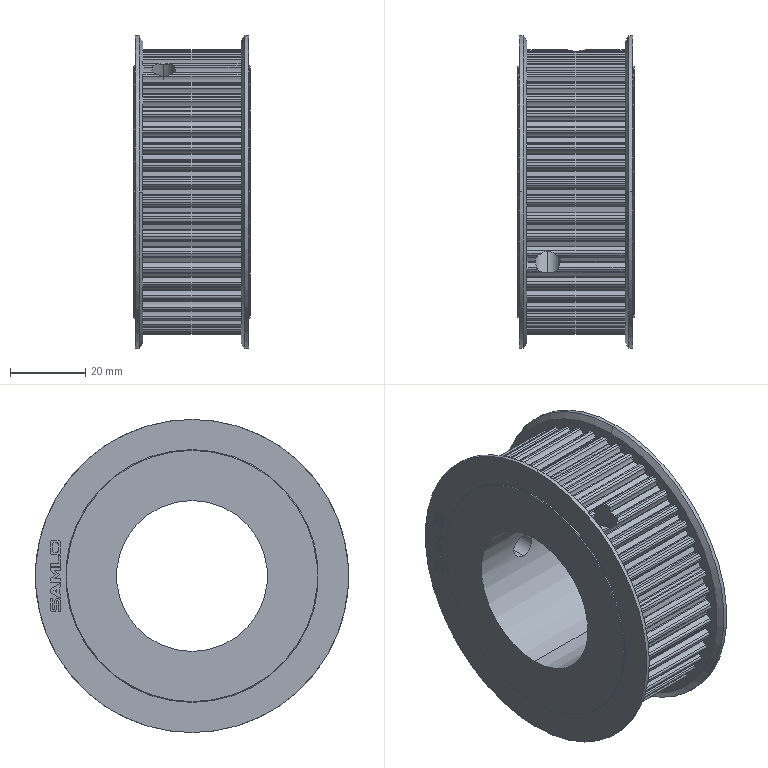Part | SolidWorks | features MoveFace 2, BaseBody 1, ICE 1 | 1 solid | 542 faces | box 31 x 83 x 83 mm | volume 94794 mm3 | cylinder 476 | plane 58 | cone 8 | commonest cylinder face diameters 1.1 x122 0.5 x115 6.55 x108 75.43 x52 71.89 x51 0.643 x4